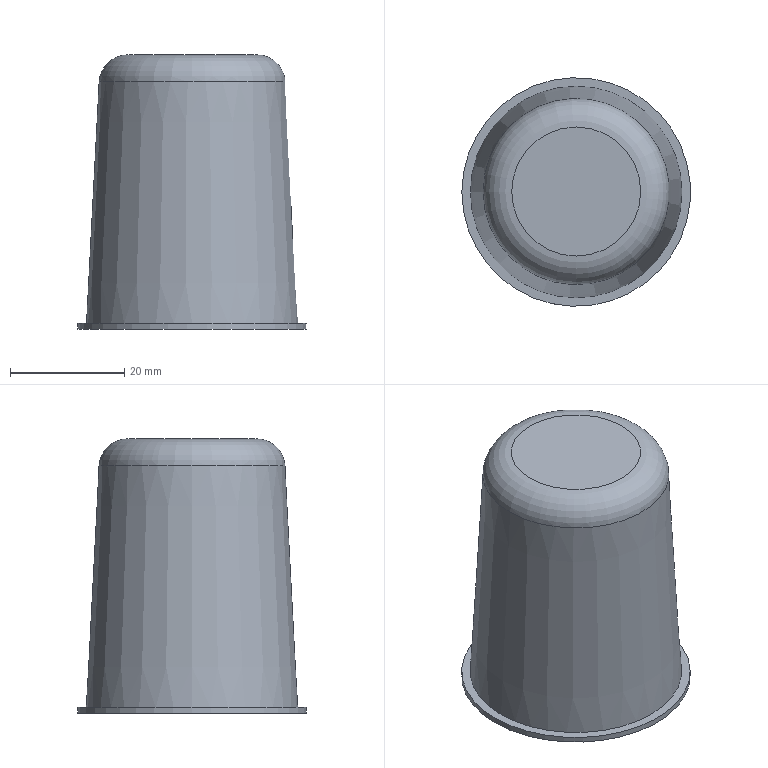Part | STEP file | CMT7E v7 | 1 solid | 6 faces | box 40 x 40 x 48 mm | volume 44913 mm3 | plane 3 | cylinder 1 | cone 1 | torus 1 | commonest cylinder face diameters 40 x1
STEP:
#1=CARTESIAN_POINT('',(0.,0.,0.));
#2=DIRECTION('',(0.,0.,1.));
#3=DIRECTION('',(1.,0.,0.));
#4=AXIS2_PLACEMENT_3D('',#1,#2,#3);
#5=CARTESIAN_POINT('',(48.,-27.,255.));
#6=VERTEX_POINT('',#5);
#7=CARTESIAN_POINT('',(68.,-27.,255.));
#8=DIRECTION('',(0.,0.,1.));
#9=DIRECTION('',(-1.,0.,0.));
#10=AXIS2_PLACEMENT_3D('',#7,#8,#9);
#11=CIRCLE('',#10,20.);
#12=CARTESIAN_POINT('',(68.,-27.,255.));
#13=DIRECTION('',(0.,0.,1.));
#14=DIRECTION('',(-1.,0.,0.));
#15=AXIS2_PLACEMENT_3D('',#12,#13,#14);
#16=PLANE('',#15);
#17=CARTESIAN_POINT('',(0.,0.));
#18=DIRECTION('',(1.,0.));
#19=AXIS2_PLACEMENT_2D('',#17,#18);
#20=CIRCLE('',#19,20.);
#21=(GEOMETRIC_REPRESENTATION_CONTEXT(2)PARAMETRIC_REPRESENTATION_CONTEXT()REPRESENTATION_CONTEXT('',''));
#22=DEFINITIONAL_REPRESENTATION('',(#20),#21);
#23=PCURVE('',#16,#22);
#24=CARTESIAN_POINT('',(68.,-27.,255.));
#25=DIRECTION('',(0.,0.,1.));
#26=DIRECTION('',(-1.,0.,0.));
#27=AXIS2_PLACEMENT_3D('',#24,#25,#26);
#28=CYLINDRICAL_SURFACE('',#27,20.);
#29=CARTESIAN_POINT('',(0.,0.));
#30=DIRECTION('',(1.,0.));
#31=VECTOR('',#30,1.);
#32=LINE('',#29,#31);
#33=(GEOMETRIC_REPRESENTATION_CONTEXT(2)PARAMETRIC_REPRESENTATION_CONTEXT()REPRESENTATION_CONTEXT('',''));
#34=DEFINITIONAL_REPRESENTATION('',(#32),#33);
#35=PCURVE('',#28,#34);
#36=SURFACE_CURVE('',#11,(#23,#35),.PCURVE_S1.);
#37=EDGE_CURVE('',#6,#6,#36,.T.);
#38=ORIENTED_EDGE('',*,*,#37,.F.);
#39=EDGE_LOOP('',(#38));
#40=FACE_BOUND('',#39,.T.);
#41=ADVANCED_FACE('',(#40),#16,.F.);
#42=CARTESIAN_POINT('',(49.5,-27.,256.));
#43=VERTEX_POINT('',#42);
#44=CARTESIAN_POINT('',(68.,-27.,256.));
#45=DIRECTION('',(0.,0.,-1.));
#46=DIRECTION('',(-1.,0.,0.));
#47=AXIS2_PLACEMENT_3D('',#44,#45,#46);
#48=CIRCLE('',#47,18.5);
#49=CARTESIAN_POINT('',(68.,-27.,256.));
#50=DIRECTION('',(0.,0.,1.));
#51=DIRECTION('',(-1.,0.,0.));
#52=AXIS2_PLACEMENT_3D('',#49,#50,#51);
#53=PLANE('',#52);
#54=CARTESIAN_POINT('',(18.5,0.));
#55=CARTESIAN_POINT('',(18.5,-32.043));
#56=CARTESIAN_POINT('',(-9.25,-16.021));
#57=CARTESIAN_POINT('',(-37.,0.));
#58=CARTESIAN_POINT('',(-9.25,16.021));
#59=CARTESIAN_POINT('',(18.5,32.043));
#60=CARTESIAN_POINT('',(18.5,0.));
#61=(BOUNDED_CURVE()B_SPLINE_CURVE(2,(#54,#55,#56,#57,#58,#59,#60),.UNSPECIFIED.,.T.,.F.)B_SPLINE_CURVE_WITH_KNOTS((1,2,2,2,2,1),(-2.094,0.,2.094,4.189,6.283,8.378),.UNSPECIFIED.)CURVE()GEOMETRIC_REPRESENTATION_ITEM()RATIONAL_B_SPLINE_CURVE((1.,0.5,1.,0.5,1.,0.5,1.))REPRESENTATION_ITEM(''));
#62=(GEOMETRIC_REPRESENTATION_CONTEXT(2)PARAMETRIC_REPRESENTATION_CONTEXT()REPRESENTATION_CONTEXT('',''));
#63=DEFINITIONAL_REPRESENTATION('',(#61),#62);
#64=PCURVE('',#53,#63);
#65=CARTESIAN_POINT('',(68.,-27.,256.));
#66=DIRECTION('',(0.,0.,-1.));
#67=DIRECTION('',(-1.,0.,0.));
#68=AXIS2_PLACEMENT_3D('',#65,#66,#67);
#69=CONICAL_SURFACE('',#68,18.5,0.05236);
#70=CARTESIAN_POINT('',(0.,0.));
#71=DIRECTION('',(1.,0.));
#72=VECTOR('',#71,1.);
#73=LINE('',#70,#72);
#74=(GEOMETRIC_REPRESENTATION_CONTEXT(2)PARAMETRIC_REPRESENTATION_CONTEXT()REPRESENTATION_CONTEXT('',''));
#75=DEFINITIONAL_REPRESENTATION('',(#73),#74);
#76=PCURVE('',#69,#75);
#77=SURFACE_CURVE('',#48,(#64,#76),.PCURVE_S1.);
#78=EDGE_CURVE('',#43,#43,#77,.T.);
#79=ORIENTED_EDGE('',*,*,#78,.T.);
#80=EDGE_LOOP('',(#79));
#81=FACE_BOUND('',#80,.T.);
#82=CARTESIAN_POINT('',(48.,-27.,256.));
#83=VERTEX_POINT('',#82);
#84=CARTESIAN_POINT('',(68.,-27.,256.));
#85=DIRECTION('',(0.,0.,1.));
#86=DIRECTION('',(-1.,0.,0.));
#87=AXIS2_PLACEMENT_3D('',#84,#85,#86);
#88=CIRCLE('',#87,20.);
#89=CARTESIAN_POINT('',(0.,0.));
#90=DIRECTION('',(1.,0.));
#91=AXIS2_PLACEMENT_2D('',#89,#90);
#92=CIRCLE('',#91,20.);
#93=(GEOMETRIC_REPRESENTATION_CONTEXT(2)PARAMETRIC_REPRESENTATION_CONTEXT()REPRESENTATION_CONTEXT('',''));
#94=DEFINITIONAL_REPRESENTATION('',(#92),#93);
#95=PCURVE('',#53,#94);
#96=CARTESIAN_POINT('',(0.,1.));
#97=DIRECTION('',(1.,0.));
#98=VECTOR('',#97,1.);
#99=LINE('',#96,#98);
#100=(GEOMETRIC_REPRESENTATION_CONTEXT(2)PARAMETRIC_REPRESENTATION_CONTEXT()REPRESENTATION_CONTEXT('',''));
#101=DEFINITIONAL_REPRESENTATION('',(#99),#100);
#102=PCURVE('',#28,#101);
#103=SURFACE_CURVE('',#88,(#95,#102),.PCURVE_S1.);
#104=EDGE_CURVE('',#83,#83,#103,.T.);
#105=ORIENTED_EDGE('',*,*,#104,.T.);
#106=EDGE_LOOP('',(#105));
#107=FACE_BOUND('',#106,.T.);
#108=ADVANCED_FACE('',(#81,#107),#53,.T.);
#109=ORIENTED_EDGE('',*,*,#37,.T.);
#110=CARTESIAN_POINT('',(48.,-27.,255.));
#111=CARTESIAN_POINT('',(48.,-27.,256.));
#112=B_SPLINE_CURVE_WITH_KNOTS('',1,(#110,#111),.UNSPECIFIED.,.F.,.F.,(2,2),(0.,1.),.PIECEWISE_BEZIER_KNOTS.);
#113=CARTESIAN_POINT('',(6.283,0.));
#114=DIRECTION('',(0.,1.));
#115=VECTOR('',#114,1.);
#116=LINE('',#113,#115);
#117=(GEOMETRIC_REPRESENTATION_CONTEXT(2)PARAMETRIC_REPRESENTATION_CONTEXT()REPRESENTATION_CONTEXT('',''));
#118=DEFINITIONAL_REPRESENTATION('',(#116),#117);
#119=PCURVE('',#28,#118);
#120=CARTESIAN_POINT('',(0.,0.));
#121=DIRECTION('',(0.,1.));
#122=VECTOR('',#121,1.);
#123=LINE('',#120,#122);
#124=(GEOMETRIC_REPRESENTATION_CONTEXT(2)PARAMETRIC_REPRESENTATION_CONTEXT()REPRESENTATION_CONTEXT('',''));
#125=DEFINITIONAL_REPRESENTATION('',(#123),#124);
#126=PCURVE('',#28,#125);
#127=SEAM_CURVE('',#112,(#119,#126),.PCURVE_S1.);
#128=EDGE_CURVE('',#6,#83,#127,.T.);
#129=ORIENTED_EDGE('',*,*,#128,.T.);
#130=ORIENTED_EDGE('',*,*,#104,.F.);
#131=ORIENTED_EDGE('',*,*,#128,.F.);
#132=EDGE_LOOP('',(#109,#129,#130,#131));
#133=FACE_BOUND('',#132,.T.);
#134=ADVANCED_FACE('',(#133),#28,.T.);
#135=CARTESIAN_POINT('',(56.708,-27.,303.));
#136=VERTEX_POINT('',#135);
#137=CARTESIAN_POINT('',(68.,-27.,303.));
#138=DIRECTION('',(0.,0.,-1.));
#139=DIRECTION('',(-1.,0.,0.));
#140=AXIS2_PLACEMENT_3D('',#137,#138,#139);
#141=CIRCLE('',#140,11.292);
#142=CARTESIAN_POINT('',(68.,-27.,303.));
#143=DIRECTION('',(0.,0.,1.));
#144=DIRECTION('',(-1.,0.,0.));
#145=AXIS2_PLACEMENT_3D('',#142,#143,#144);
#146=PLANE('',#145);
#147=CARTESIAN_POINT('',(11.292,0.));
#148=CARTESIAN_POINT('',(11.292,-19.558));
#149=CARTESIAN_POINT('',(-5.646,-9.779));
#150=CARTESIAN_POINT('',(-22.584,0.));
#151=CARTESIAN_POINT('',(-5.646,9.779));
#152=CARTESIAN_POINT('',(11.292,19.558));
#153=CARTESIAN_POINT('',(11.292,0.));
#154=(BOUNDED_CURVE()B_SPLINE_CURVE(2,(#147,#148,#149,#150,#151,#152,#153),.UNSPECIFIED.,.T.,.F.)B_SPLINE_CURVE_WITH_KNOTS((1,2,2,2,2,1),(-2.094,0.,2.094,4.189,6.283,8.378),.UNSPECIFIED.)CURVE()GEOMETRIC_REPRESENTATION_ITEM()RATIONAL_B_SPLINE_CURVE((1.,0.5,1.,0.5,1.,0.5,1.))REPRESENTATION_ITEM(''));
#155=(GEOMETRIC_REPRESENTATION_CONTEXT(2)PARAMETRIC_REPRESENTATION_CONTEXT()REPRESENTATION_CONTEXT('',''));
#156=DEFINITIONAL_REPRESENTATION('',(#154),#155);
#157=PCURVE('',#146,#156);
#158=CARTESIAN_POINT('',(68.,-27.,298.));
#159=DIRECTION('',(0.,0.,-1.));
#160=DIRECTION('',(-1.,0.,0.));
#161=AXIS2_PLACEMENT_3D('',#158,#159,#160);
#162=TOROIDAL_SURFACE('',#161,11.292,5.);
#163=CARTESIAN_POINT('',(0.,4.712));
#164=DIRECTION('',(1.,0.));
#165=VECTOR('',#164,1.);
#166=LINE('',#163,#165);
#167=(GEOMETRIC_REPRESENTATION_CONTEXT(2)PARAMETRIC_REPRESENTATION_CONTEXT()REPRESENTATION_CONTEXT('',''));
#168=DEFINITIONAL_REPRESENTATION('',(#166),#167);
#169=PCURVE('',#162,#168);
#170=SURFACE_CURVE('',#141,(#157,#169),.PCURVE_S1.);
#171=EDGE_CURVE('',#136,#136,#170,.T.);
#172=ORIENTED_EDGE('',*,*,#171,.F.);
#173=EDGE_LOOP('',(#172));
#174=FACE_BOUND('',#173,.T.);
#175=ADVANCED_FACE('',(#174),#146,.T.);
#176=ORIENTED_EDGE('',*,*,#78,.F.);
#177=CARTESIAN_POINT('',(51.715,-27.,298.262));
#178=VERTEX_POINT('',#177);
#179=CARTESIAN_POINT('',(51.715,-27.,298.262));
#180=CARTESIAN_POINT('',(49.5,-27.,256.));
#181=B_SPLINE_CURVE_WITH_KNOTS('',1,(#179,#180),.UNSPECIFIED.,.F.,.F.,(2,2),(-42.32,0.),.PIECEWISE_BEZIER_KNOTS.);
#182=CARTESIAN_POINT('',(0.,0.));
#183=DIRECTION('',(0.,1.));
#184=VECTOR('',#183,1.);
#185=LINE('',#182,#184);
#186=(GEOMETRIC_REPRESENTATION_CONTEXT(2)PARAMETRIC_REPRESENTATION_CONTEXT()REPRESENTATION_CONTEXT('',''));
#187=DEFINITIONAL_REPRESENTATION('',(#185),#186);
#188=PCURVE('',#69,#187);
#189=CARTESIAN_POINT('',(6.283,0.));
#190=DIRECTION('',(0.,1.));
#191=VECTOR('',#190,1.);
#192=LINE('',#189,#191);
#193=(GEOMETRIC_REPRESENTATION_CONTEXT(2)PARAMETRIC_REPRESENTATION_CONTEXT()REPRESENTATION_CONTEXT('',''));
#194=DEFINITIONAL_REPRESENTATION('',(#192),#193);
#195=PCURVE('',#69,#194);
#196=SEAM_CURVE('',#181,(#188,#195),.PCURVE_S1.);
#197=EDGE_CURVE('',#178,#43,#196,.T.);
#198=ORIENTED_EDGE('',*,*,#197,.F.);
#199=CARTESIAN_POINT('',(68.,-27.,298.262));
#200=DIRECTION('',(0.,0.,1.));
#201=DIRECTION('',(-1.,0.,0.));
#202=AXIS2_PLACEMENT_3D('',#199,#200,#201);
#203=CIRCLE('',#202,16.285);
#204=CARTESIAN_POINT('',(6.283,-42.262));
#205=DIRECTION('',(-1.,0.));
#206=VECTOR('',#205,1.);
#207=LINE('',#204,#206);
#208=(GEOMETRIC_REPRESENTATION_CONTEXT(2)PARAMETRIC_REPRESENTATION_CONTEXT()REPRESENTATION_CONTEXT('',''));
#209=DEFINITIONAL_REPRESENTATION('',(#207),#208);
#210=PCURVE('',#69,#209);
#211=CARTESIAN_POINT('',(6.283,6.231));
#212=DIRECTION('',(-1.,0.));
#213=VECTOR('',#212,1.);
#214=LINE('',#211,#213);
#215=(GEOMETRIC_REPRESENTATION_CONTEXT(2)PARAMETRIC_REPRESENTATION_CONTEXT()REPRESENTATION_CONTEXT('',''));
#216=DEFINITIONAL_REPRESENTATION('',(#214),#215);
#217=PCURVE('',#162,#216);
#218=SURFACE_CURVE('',#203,(#210,#217),.PCURVE_S1.);
#219=EDGE_CURVE('',#178,#178,#218,.T.);
#220=ORIENTED_EDGE('',*,*,#219,.F.);
#221=ORIENTED_EDGE('',*,*,#197,.T.);
#222=EDGE_LOOP('',(#176,#198,#220,#221));
#223=FACE_BOUND('',#222,.T.);
#224=ADVANCED_FACE('',(#223),#69,.T.);
#225=ORIENTED_EDGE('',*,*,#171,.T.);
#226=CARTESIAN_POINT('',(56.708,-27.,303.));
#227=CARTESIAN_POINT('',(55.418,-27.,303.));
#228=CARTESIAN_POINT('',(54.159,-27.,302.604));
#229=CARTESIAN_POINT('',(53.063,-27.,301.841));
#230=CARTESIAN_POINT('',(52.244,-27.,300.787));
#231=CARTESIAN_POINT('',(51.782,-27.,299.55));
#232=CARTESIAN_POINT('',(51.715,-27.,298.262));
#233=(BOUNDED_CURVE()B_SPLINE_CURVE(6,(#226,#227,#228,#229,#230,#231,#232),.UNSPECIFIED.,.F.,.F.)B_SPLINE_CURVE_WITH_KNOTS((7,7),(4.712,6.231),.PIECEWISE_BEZIER_KNOTS.)CURVE()GEOMETRIC_REPRESENTATION_ITEM()RATIONAL_B_SPLINE_CURVE((1.029,1.009,0.9981,0.9943,0.9981,1.009,1.029))REPRESENTATION_ITEM(''));
#234=CARTESIAN_POINT('',(6.283,0.));
#235=DIRECTION('',(0.,1.));
#236=VECTOR('',#235,1.);
#237=LINE('',#234,#236);
#238=(GEOMETRIC_REPRESENTATION_CONTEXT(2)PARAMETRIC_REPRESENTATION_CONTEXT()REPRESENTATION_CONTEXT('',''));
#239=DEFINITIONAL_REPRESENTATION('',(#237),#238);
#240=PCURVE('',#162,#239);
#241=CARTESIAN_POINT('',(0.,0.));
#242=DIRECTION('',(0.,1.));
#243=VECTOR('',#242,1.);
#244=LINE('',#241,#243);
#245=(GEOMETRIC_REPRESENTATION_CONTEXT(2)PARAMETRIC_REPRESENTATION_CONTEXT()REPRESENTATION_CONTEXT('',''));
#246=DEFINITIONAL_REPRESENTATION('',(#244),#245);
#247=PCURVE('',#162,#246);
#248=SEAM_CURVE('',#233,(#240,#247),.PCURVE_S1.);
#249=EDGE_CURVE('',#136,#178,#248,.T.);
#250=ORIENTED_EDGE('',*,*,#249,.T.);
#251=ORIENTED_EDGE('',*,*,#219,.T.);
#252=ORIENTED_EDGE('',*,*,#249,.F.);
#253=EDGE_LOOP('',(#225,#250,#251,#252));
#254=FACE_BOUND('',#253,.T.);
#255=ADVANCED_FACE('',(#254),#162,.T.);
#256=CLOSED_SHELL('',(#41,#108,#134,#175,#224,#255));
#257=MANIFOLD_SOLID_BREP('',#256);
#258=(LENGTH_UNIT()NAMED_UNIT(*)SI_UNIT(.MILLI.,.METRE.));
#259=UNCERTAINTY_MEASURE_WITH_UNIT(LENGTH_MEASURE(0.0000002),#258,'','');
#260=(NAMED_UNIT(*)PLANE_ANGLE_UNIT()SI_UNIT($,.RADIAN.));
#261=(NAMED_UNIT(*)SI_UNIT($,.STERADIAN.)SOLID_ANGLE_UNIT());
#262=(GEOMETRIC_REPRESENTATION_CONTEXT(3)GLOBAL_UNCERTAINTY_ASSIGNED_CONTEXT((#259))GLOBAL_UNIT_ASSIGNED_CONTEXT((#258,#260,#261))REPRESENTATION_CONTEXT('',''));
#263=ADVANCED_BREP_SHAPE_REPRESENTATION('',(#4,#257),#262);